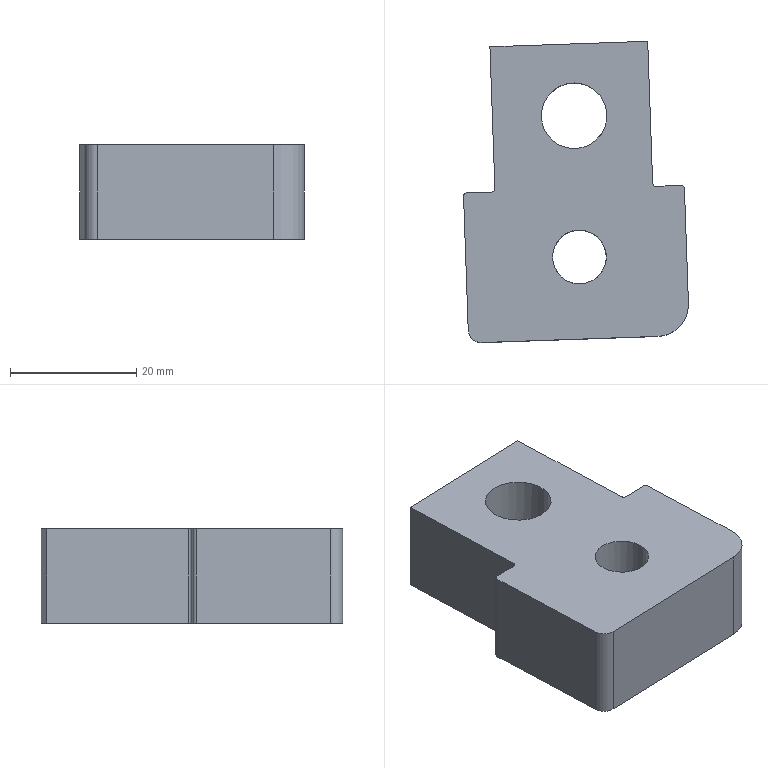Part | NX | features PS-30 2 | 1 solid | 18 faces | box 35.619 x 47.713 x 15 mm | volume 18881 mm3 | plane 10 | cylinder 8 | commonest cylinder face diameters 1 x4 4 x1 8.506 x1 10 x1 10.4 x1
STEP:
#1=CARTESIAN_POINT('',(3332.266,-814.738,900.716));
#2=VERTEX_POINT('',#1);
#3=CARTESIAN_POINT('',(3332.266,-809.538,900.716));
#4=DIRECTION('',(0.,0.,1.));
#5=DIRECTION('',(0.,-1.,0.));
#6=AXIS2_PLACEMENT_3D('',#3,#4,#5);
#7=CIRCLE('',#6,5.2);
#8=EDGE_CURVE('',#2,#2,#7,.F.);
#9=ORIENTED_EDGE('',*,*,#8,.F.);
#10=EDGE_LOOP('',(#9));
#11=FACE_BOUND('',#10,.T.);
#12=CARTESIAN_POINT('',(3327.066,-809.538,885.716));
#13=VERTEX_POINT('',#12);
#14=CARTESIAN_POINT('',(3332.266,-809.538,885.716));
#15=DIRECTION('',(0.,0.,-1.));
#16=DIRECTION('',(-1.,0.,0.));
#17=AXIS2_PLACEMENT_3D('',#14,#15,#16);
#18=CIRCLE('',#17,5.2);
#19=EDGE_CURVE('',#13,#13,#18,.F.);
#20=ORIENTED_EDGE('',*,*,#19,.F.);
#21=EDGE_LOOP('',(#20));
#22=FACE_BOUND('',#21,.T.);
#23=CARTESIAN_POINT('',(3332.266,-809.538,890.716));
#24=DIRECTION('',(0.,0.,-1.));
#25=DIRECTION('',(0.9976,0.06975,0.));
#26=AXIS2_PLACEMENT_3D('',#23,#24,#25);
#27=CYLINDRICAL_SURFACE('',#26,5.2);
#28=ADVANCED_FACE('',(#11,#22),#27,.F.);
#29=CARTESIAN_POINT('',(3333.107,-836.157,900.716));
#30=VERTEX_POINT('',#29);
#31=CARTESIAN_POINT('',(3333.107,-831.904,900.716));
#32=DIRECTION('',(0.,0.,1.));
#33=DIRECTION('',(0.,-1.,0.));
#34=AXIS2_PLACEMENT_3D('',#31,#32,#33);
#35=CIRCLE('',#34,4.253);
#36=EDGE_CURVE('',#30,#30,#35,.F.);
#37=ORIENTED_EDGE('',*,*,#36,.F.);
#38=EDGE_LOOP('',(#37));
#39=FACE_BOUND('',#38,.T.);
#40=CARTESIAN_POINT('',(3328.854,-831.904,885.716));
#41=VERTEX_POINT('',#40);
#42=CARTESIAN_POINT('',(3333.107,-831.904,885.716));
#43=DIRECTION('',(0.,0.,-1.));
#44=DIRECTION('',(-1.,0.,0.));
#45=AXIS2_PLACEMENT_3D('',#42,#43,#44);
#46=CIRCLE('',#45,4.253);
#47=EDGE_CURVE('',#41,#41,#46,.T.);
#48=ORIENTED_EDGE('',*,*,#47,.T.);
#49=EDGE_LOOP('',(#48));
#50=FACE_BOUND('',#49,.T.);
#51=CARTESIAN_POINT('',(3333.107,-831.904,868.716));
#52=DIRECTION('',(0.,0.,1.));
#53=DIRECTION('',(0.9976,0.06975,0.));
#54=AXIS2_PLACEMENT_3D('',#51,#52,#53);
#55=CYLINDRICAL_SURFACE('',#54,4.253);
#56=ADVANCED_FACE('',(#39,#50),#55,.F.);
#57=ORIENTED_EDGE('',*,*,#36,.T.);
#58=EDGE_LOOP('',(#57));
#59=FACE_BOUND('',#58,.T.);
#60=CARTESIAN_POINT('',(3319.24,-821.618,900.716));
#61=VERTEX_POINT('',#60);
#62=CARTESIAN_POINT('',(3319.722,-821.101,900.716));
#63=VERTEX_POINT('',#62);
#64=CARTESIAN_POINT('',(3319.222,-821.119,900.716));
#65=DIRECTION('',(0.,0.,1.));
#66=DIRECTION('',(0.,-1.,0.));
#67=AXIS2_PLACEMENT_3D('',#64,#65,#66);
#68=CIRCLE('',#67,0.5);
#69=EDGE_CURVE('',#61,#63,#68,.T.);
#70=ORIENTED_EDGE('',*,*,#69,.F.);
#71=CARTESIAN_POINT('',(3315.242,-821.758,900.716));
#72=VERTEX_POINT('',#71);
#73=CARTESIAN_POINT('',(3173.832,-826.696,900.716));
#74=DIRECTION('',(0.9994,0.0349,0.));
#75=VECTOR('',#74,1000.);
#76=LINE('',#73,#75);
#77=EDGE_CURVE('',#61,#72,#76,.F.);
#78=ORIENTED_EDGE('',*,*,#77,.T.);
#79=CARTESIAN_POINT('',(3314.76,-822.275,900.716));
#80=VERTEX_POINT('',#79);
#81=CARTESIAN_POINT('',(3315.26,-822.258,900.716));
#82=DIRECTION('',(0.,0.,1.));
#83=DIRECTION('',(0.,-1.,0.));
#84=AXIS2_PLACEMENT_3D('',#81,#82,#83);
#85=CIRCLE('',#84,0.5);
#86=EDGE_CURVE('',#80,#72,#85,.F.);
#87=ORIENTED_EDGE('',*,*,#86,.F.);
#88=CARTESIAN_POINT('',(3315.502,-843.525,900.716));
#89=VERTEX_POINT('',#88);
#90=CARTESIAN_POINT('',(3312.834,-767.126,900.716));
#91=DIRECTION('',(-0.0349,0.9994,0.));
#92=VECTOR('',#91,1000.);
#93=LINE('',#90,#92);
#94=EDGE_CURVE('',#80,#89,#93,.F.);
#95=ORIENTED_EDGE('',*,*,#94,.T.);
#96=CARTESIAN_POINT('',(3317.57,-845.454,900.716));
#97=VERTEX_POINT('',#96);
#98=CARTESIAN_POINT('',(3317.501,-843.455,900.716));
#99=DIRECTION('',(0.,0.,1.));
#100=DIRECTION('',(0.,-1.,0.));
#101=AXIS2_PLACEMENT_3D('',#98,#99,#100);
#102=CIRCLE('',#101,2.);
#103=EDGE_CURVE('',#89,#97,#102,.T.);
#104=ORIENTED_EDGE('',*,*,#103,.T.);
#105=CARTESIAN_POINT('',(3345.553,-844.477,900.716));
#106=VERTEX_POINT('',#105);
#107=CARTESIAN_POINT('',(3174.662,-850.444,900.716));
#108=DIRECTION('',(-0.9994,-0.0349,0.));
#109=VECTOR('',#108,1000.);
#110=LINE('',#107,#109);
#111=EDGE_CURVE('',#106,#97,#110,.T.);
#112=ORIENTED_EDGE('',*,*,#111,.F.);
#113=CARTESIAN_POINT('',(3350.376,-839.306,900.716));
#114=VERTEX_POINT('',#113);
#115=CARTESIAN_POINT('',(3345.379,-839.48,900.716));
#116=DIRECTION('',(0.,0.,1.));
#117=DIRECTION('',(0.,-1.,0.));
#118=AXIS2_PLACEMENT_3D('',#115,#116,#117);
#119=CIRCLE('',#118,5.);
#120=EDGE_CURVE('',#106,#114,#119,.T.);
#121=ORIENTED_EDGE('',*,*,#120,.T.);
#122=CARTESIAN_POINT('',(3349.739,-821.054,900.716));
#123=VERTEX_POINT('',#122);
#124=CARTESIAN_POINT('',(3347.813,-765.904,900.716));
#125=DIRECTION('',(-0.0349,0.9994,0.));
#126=VECTOR('',#125,1000.);
#127=LINE('',#124,#126);
#128=EDGE_CURVE('',#123,#114,#127,.F.);
#129=ORIENTED_EDGE('',*,*,#128,.F.);
#130=CARTESIAN_POINT('',(3349.221,-820.572,900.716));
#131=VERTEX_POINT('',#130);
#132=CARTESIAN_POINT('',(3349.239,-821.071,900.716));
#133=DIRECTION('',(0.,0.,1.));
#134=DIRECTION('',(0.,-1.,0.));
#135=AXIS2_PLACEMENT_3D('',#132,#133,#134);
#136=CIRCLE('',#135,0.5);
#137=EDGE_CURVE('',#131,#123,#136,.F.);
#138=ORIENTED_EDGE('',*,*,#137,.F.);
#139=CARTESIAN_POINT('',(3345.224,-820.711,900.716));
#140=VERTEX_POINT('',#139);
#141=CARTESIAN_POINT('',(3173.832,-826.696,900.716));
#142=DIRECTION('',(0.9994,0.0349,0.));
#143=VECTOR('',#142,1000.);
#144=LINE('',#141,#143);
#145=EDGE_CURVE('',#131,#140,#144,.F.);
#146=ORIENTED_EDGE('',*,*,#145,.T.);
#147=CARTESIAN_POINT('',(3344.707,-820.229,900.716));
#148=VERTEX_POINT('',#147);
#149=CARTESIAN_POINT('',(3345.206,-820.211,900.716));
#150=DIRECTION('',(0.,0.,1.));
#151=DIRECTION('',(0.,-1.,0.));
#152=AXIS2_PLACEMENT_3D('',#149,#150,#151);
#153=CIRCLE('',#152,0.5);
#154=EDGE_CURVE('',#148,#140,#153,.T.);
#155=ORIENTED_EDGE('',*,*,#154,.F.);
#156=CARTESIAN_POINT('',(3343.922,-797.743,900.716));
#157=VERTEX_POINT('',#156);
#158=CARTESIAN_POINT('',(3342.816,-766.079,900.716));
#159=DIRECTION('',(-0.0349,0.9994,0.));
#160=VECTOR('',#159,1000.);
#161=LINE('',#158,#160);
#162=EDGE_CURVE('',#157,#148,#161,.F.);
#163=ORIENTED_EDGE('',*,*,#162,.F.);
#164=CARTESIAN_POINT('',(3318.937,-798.615,900.716));
#165=VERTEX_POINT('',#164);
#166=CARTESIAN_POINT('',(3328.742,-798.273,900.716));
#167=DIRECTION('',(-0.9994,-0.0349,0.));
#168=VECTOR('',#167,1000.);
#169=LINE('',#166,#168);
#170=EDGE_CURVE('',#157,#165,#169,.T.);
#171=ORIENTED_EDGE('',*,*,#170,.T.);
#172=CARTESIAN_POINT('',(3317.831,-766.951,900.716));
#173=DIRECTION('',(-0.0349,0.9994,0.));
#174=VECTOR('',#173,1000.);
#175=LINE('',#172,#174);
#176=EDGE_CURVE('',#165,#63,#175,.F.);
#177=ORIENTED_EDGE('',*,*,#176,.T.);
#178=EDGE_LOOP('',(#70,#78,#87,#95,#104,#112,#121,#129,#138,#146,#155,#163,#171,#177));
#179=FACE_BOUND('',#178,.T.);
#180=ORIENTED_EDGE('',*,*,#8,.T.);
#181=EDGE_LOOP('',(#180));
#182=FACE_BOUND('',#181,.T.);
#183=CARTESIAN_POINT('',(3171.924,-772.046,900.716));
#184=DIRECTION('',(0.,0.,1.));
#185=DIRECTION('',(0.9976,0.06975,0.));
#186=AXIS2_PLACEMENT_3D('',#183,#184,#185);
#187=PLANE('',#186);
#188=ADVANCED_FACE('',(#59,#179,#182),#187,.T.);
#189=CARTESIAN_POINT('',(3349.739,-821.054,885.716));
#190=VERTEX_POINT('',#189);
#191=CARTESIAN_POINT('',(3349.739,-821.054,868.716));
#192=DIRECTION('',(0.,0.,-1.));
#193=VECTOR('',#192,1000.);
#194=LINE('',#191,#193);
#195=EDGE_CURVE('',#123,#190,#194,.T.);
#196=ORIENTED_EDGE('',*,*,#195,.T.);
#197=CARTESIAN_POINT('',(3349.221,-820.572,885.716));
#198=VERTEX_POINT('',#197);
#199=CARTESIAN_POINT('',(3349.239,-821.071,885.716));
#200=DIRECTION('',(0.,0.,-1.));
#201=DIRECTION('',(-1.,0.,0.));
#202=AXIS2_PLACEMENT_3D('',#199,#200,#201);
#203=CIRCLE('',#202,0.5);
#204=EDGE_CURVE('',#190,#198,#203,.F.);
#205=ORIENTED_EDGE('',*,*,#204,.T.);
#206=CARTESIAN_POINT('',(3349.221,-820.572,890.716));
#207=DIRECTION('',(0.,0.,-1.));
#208=VECTOR('',#207,1000.);
#209=LINE('',#206,#208);
#210=EDGE_CURVE('',#198,#131,#209,.F.);
#211=ORIENTED_EDGE('',*,*,#210,.T.);
#212=ORIENTED_EDGE('',*,*,#137,.T.);
#213=EDGE_LOOP('',(#196,#205,#211,#212));
#214=FACE_BOUND('',#213,.T.);
#215=CARTESIAN_POINT('',(3349.239,-821.071,862.716));
#216=DIRECTION('',(0.,0.,1.));
#217=DIRECTION('',(1.,0.,0.));
#218=AXIS2_PLACEMENT_3D('',#215,#216,#217);
#219=CYLINDRICAL_SURFACE('',#218,0.5);
#220=ADVANCED_FACE('',(#214),#219,.T.);
#221=CARTESIAN_POINT('',(3345.553,-844.477,885.716));
#222=VERTEX_POINT('',#221);
#223=CARTESIAN_POINT('',(3345.553,-844.477,935.716));
#224=DIRECTION('',(0.,0.,-1.));
#225=VECTOR('',#224,1000.);
#226=LINE('',#223,#225);
#227=EDGE_CURVE('',#222,#106,#226,.F.);
#228=ORIENTED_EDGE('',*,*,#227,.F.);
#229=CARTESIAN_POINT('',(3350.376,-839.306,885.716));
#230=VERTEX_POINT('',#229);
#231=CARTESIAN_POINT('',(3345.379,-839.48,885.716));
#232=DIRECTION('',(0.,0.,-1.));
#233=DIRECTION('',(-1.,0.,0.));
#234=AXIS2_PLACEMENT_3D('',#231,#232,#233);
#235=CIRCLE('',#234,5.);
#236=EDGE_CURVE('',#230,#222,#235,.T.);
#237=ORIENTED_EDGE('',*,*,#236,.F.);
#238=CARTESIAN_POINT('',(3350.376,-839.306,862.716));
#239=DIRECTION('',(0.,0.,1.));
#240=VECTOR('',#239,1000.);
#241=LINE('',#238,#240);
#242=EDGE_CURVE('',#114,#230,#241,.F.);
#243=ORIENTED_EDGE('',*,*,#242,.F.);
#244=ORIENTED_EDGE('',*,*,#120,.F.);
#245=EDGE_LOOP('',(#228,#237,#243,#244));
#246=FACE_BOUND('',#245,.T.);
#247=CARTESIAN_POINT('',(3345.379,-839.48,862.716));
#248=DIRECTION('',(0.,0.,1.));
#249=DIRECTION('',(0.9976,0.06975,0.));
#250=AXIS2_PLACEMENT_3D('',#247,#248,#249);
#251=CYLINDRICAL_SURFACE('',#250,5.);
#252=ADVANCED_FACE('',(#246),#251,.T.);
#253=CARTESIAN_POINT('',(3315.242,-821.758,885.716));
#254=VERTEX_POINT('',#253);
#255=CARTESIAN_POINT('',(3315.242,-821.758,863.216));
#256=DIRECTION('',(0.,0.,1.));
#257=VECTOR('',#256,1000.);
#258=LINE('',#255,#257);
#259=EDGE_CURVE('',#72,#254,#258,.F.);
#260=ORIENTED_EDGE('',*,*,#259,.T.);
#261=CARTESIAN_POINT('',(3314.76,-822.275,885.716));
#262=VERTEX_POINT('',#261);
#263=CARTESIAN_POINT('',(3315.26,-822.258,885.716));
#264=DIRECTION('',(0.,0.,-1.));
#265=DIRECTION('',(-1.,0.,0.));
#266=AXIS2_PLACEMENT_3D('',#263,#264,#265);
#267=CIRCLE('',#266,0.5);
#268=EDGE_CURVE('',#262,#254,#267,.T.);
#269=ORIENTED_EDGE('',*,*,#268,.F.);
#270=CARTESIAN_POINT('',(3314.76,-822.275,890.716));
#271=DIRECTION('',(0.,0.,1.));
#272=VECTOR('',#271,1000.);
#273=LINE('',#270,#272);
#274=EDGE_CURVE('',#262,#80,#273,.T.);
#275=ORIENTED_EDGE('',*,*,#274,.T.);
#276=ORIENTED_EDGE('',*,*,#86,.T.);
#277=EDGE_LOOP('',(#260,#269,#275,#276));
#278=FACE_BOUND('',#277,.T.);
#279=CARTESIAN_POINT('',(3315.26,-822.258,890.716));
#280=DIRECTION('',(0.,0.,1.));
#281=DIRECTION('',(1.,0.,0.));
#282=AXIS2_PLACEMENT_3D('',#279,#280,#281);
#283=CYLINDRICAL_SURFACE('',#282,0.5);
#284=ADVANCED_FACE('',(#278),#283,.T.);
#285=CARTESIAN_POINT('',(3315.502,-843.525,885.716));
#286=VERTEX_POINT('',#285);
#287=CARTESIAN_POINT('',(3315.502,-843.525,890.716));
#288=DIRECTION('',(0.,0.,1.));
#289=VECTOR('',#288,1000.);
#290=LINE('',#287,#289);
#291=EDGE_CURVE('',#286,#89,#290,.T.);
#292=ORIENTED_EDGE('',*,*,#291,.F.);
#293=CARTESIAN_POINT('',(3317.57,-845.454,885.716));
#294=VERTEX_POINT('',#293);
#295=CARTESIAN_POINT('',(3317.501,-843.455,885.716));
#296=DIRECTION('',(0.,0.,-1.));
#297=DIRECTION('',(-1.,0.,0.));
#298=AXIS2_PLACEMENT_3D('',#295,#296,#297);
#299=CIRCLE('',#298,2.);
#300=EDGE_CURVE('',#286,#294,#299,.F.);
#301=ORIENTED_EDGE('',*,*,#300,.T.);
#302=CARTESIAN_POINT('',(3317.57,-845.454,860.716));
#303=DIRECTION('',(0.,0.,-1.));
#304=VECTOR('',#303,1000.);
#305=LINE('',#302,#304);
#306=EDGE_CURVE('',#97,#294,#305,.T.);
#307=ORIENTED_EDGE('',*,*,#306,.F.);
#308=ORIENTED_EDGE('',*,*,#103,.F.);
#309=EDGE_LOOP('',(#292,#301,#307,#308));
#310=FACE_BOUND('',#309,.T.);
#311=CARTESIAN_POINT('',(3317.501,-843.455,935.716));
#312=DIRECTION('',(0.,0.,-1.));
#313=DIRECTION('',(-0.9976,-0.06975,0.));
#314=AXIS2_PLACEMENT_3D('',#311,#312,#313);
#315=CYLINDRICAL_SURFACE('',#314,2.);
#316=ADVANCED_FACE('',(#310),#315,.T.);
#317=CARTESIAN_POINT('',(3314.523,-815.501,885.716));
#318=DIRECTION('',(-0.0349,0.9994,0.));
#319=VECTOR('',#318,1000.);
#320=LINE('',#317,#319);
#321=EDGE_CURVE('',#262,#286,#320,.F.);
#322=ORIENTED_EDGE('',*,*,#321,.T.);
#323=ORIENTED_EDGE('',*,*,#291,.T.);
#324=ORIENTED_EDGE('',*,*,#94,.F.);
#325=ORIENTED_EDGE('',*,*,#274,.F.);
#326=EDGE_LOOP('',(#322,#323,#324,#325));
#327=FACE_BOUND('',#326,.T.);
#328=CARTESIAN_POINT('',(3314.523,-815.501,890.716));
#329=DIRECTION('',(0.9994,0.0349,0.));
#330=DIRECTION('',(-0.0349,0.9994,0.));
#331=AXIS2_PLACEMENT_3D('',#328,#329,#330);
#332=PLANE('',#331);
#333=ADVANCED_FACE('',(#327),#332,.F.);
#334=ORIENTED_EDGE('',*,*,#306,.T.);
#335=CARTESIAN_POINT('',(3304.578,-845.908,885.716));
#336=DIRECTION('',(-0.9994,-0.0349,0.));
#337=VECTOR('',#336,1000.);
#338=LINE('',#335,#337);
#339=EDGE_CURVE('',#222,#294,#338,.T.);
#340=ORIENTED_EDGE('',*,*,#339,.F.);
#341=ORIENTED_EDGE('',*,*,#227,.T.);
#342=ORIENTED_EDGE('',*,*,#111,.T.);
#343=EDGE_LOOP('',(#334,#340,#341,#342));
#344=FACE_BOUND('',#343,.T.);
#345=CARTESIAN_POINT('',(3304.578,-845.908,935.716));
#346=DIRECTION('',(-0.0349,0.9994,0.));
#347=DIRECTION('',(-0.9994,-0.0349,0.));
#348=AXIS2_PLACEMENT_3D('',#345,#346,#347);
#349=PLANE('',#348);
#350=ADVANCED_FACE('',(#344),#349,.F.);
#351=ORIENTED_EDGE('',*,*,#242,.T.);
#352=CARTESIAN_POINT('',(3349.537,-815.279,885.716));
#353=DIRECTION('',(-0.0349,0.9994,0.));
#354=VECTOR('',#353,1000.);
#355=LINE('',#352,#354);
#356=EDGE_CURVE('',#230,#190,#355,.T.);
#357=ORIENTED_EDGE('',*,*,#356,.T.);
#358=ORIENTED_EDGE('',*,*,#195,.F.);
#359=ORIENTED_EDGE('',*,*,#128,.T.);
#360=EDGE_LOOP('',(#351,#357,#358,#359));
#361=FACE_BOUND('',#360,.T.);
#362=CARTESIAN_POINT('',(3349.537,-815.279,862.716));
#363=DIRECTION('',(0.9994,0.0349,0.));
#364=DIRECTION('',(-0.0349,0.9994,0.));
#365=AXIS2_PLACEMENT_3D('',#362,#363,#364);
#366=PLANE('',#365);
#367=ADVANCED_FACE('',(#361),#366,.T.);
#368=CARTESIAN_POINT('',(3345.224,-820.711,885.716));
#369=VERTEX_POINT('',#368);
#370=CARTESIAN_POINT('',(3329.542,-821.259,885.716));
#371=DIRECTION('',(0.9994,0.0349,0.));
#372=VECTOR('',#371,1000.);
#373=LINE('',#370,#372);
#374=EDGE_CURVE('',#369,#198,#373,.T.);
#375=ORIENTED_EDGE('',*,*,#374,.F.);
#376=CARTESIAN_POINT('',(3345.224,-820.711,863.216));
#377=DIRECTION('',(0.,0.,1.));
#378=VECTOR('',#377,1000.);
#379=LINE('',#376,#378);
#380=EDGE_CURVE('',#140,#369,#379,.F.);
#381=ORIENTED_EDGE('',*,*,#380,.F.);
#382=ORIENTED_EDGE('',*,*,#145,.F.);
#383=ORIENTED_EDGE('',*,*,#210,.F.);
#384=EDGE_LOOP('',(#375,#381,#382,#383));
#385=FACE_BOUND('',#384,.T.);
#386=CARTESIAN_POINT('',(3329.542,-821.259,863.216));
#387=DIRECTION('',(0.0349,-0.9994,0.));
#388=DIRECTION('',(-0.9994,-0.0349,0.));
#389=AXIS2_PLACEMENT_3D('',#386,#387,#388);
#390=PLANE('',#389);
#391=ADVANCED_FACE('',(#385),#390,.F.);
#392=CARTESIAN_POINT('',(3319.24,-821.618,885.716));
#393=VERTEX_POINT('',#392);
#394=CARTESIAN_POINT('',(3329.542,-821.259,885.716));
#395=DIRECTION('',(0.9994,0.0349,0.));
#396=VECTOR('',#395,1000.);
#397=LINE('',#394,#396);
#398=EDGE_CURVE('',#254,#393,#397,.T.);
#399=ORIENTED_EDGE('',*,*,#398,.F.);
#400=ORIENTED_EDGE('',*,*,#259,.F.);
#401=ORIENTED_EDGE('',*,*,#77,.F.);
#402=CARTESIAN_POINT('',(3319.24,-821.618,890.716));
#403=DIRECTION('',(0.,0.,-1.));
#404=VECTOR('',#403,1000.);
#405=LINE('',#402,#404);
#406=EDGE_CURVE('',#393,#61,#405,.F.);
#407=ORIENTED_EDGE('',*,*,#406,.F.);
#408=EDGE_LOOP('',(#399,#400,#401,#407));
#409=FACE_BOUND('',#408,.T.);
#410=CARTESIAN_POINT('',(3329.542,-821.259,863.216));
#411=DIRECTION('',(0.0349,-0.9994,0.));
#412=DIRECTION('',(-0.9994,-0.0349,0.));
#413=AXIS2_PLACEMENT_3D('',#410,#411,#412);
#414=PLANE('',#413);
#415=ADVANCED_FACE('',(#409),#414,.F.);
#416=CARTESIAN_POINT('',(3344.707,-820.229,885.716));
#417=VERTEX_POINT('',#416);
#418=CARTESIAN_POINT('',(3345.206,-820.211,885.716));
#419=DIRECTION('',(0.,0.,-1.));
#420=DIRECTION('',(-1.,0.,0.));
#421=AXIS2_PLACEMENT_3D('',#418,#419,#420);
#422=CIRCLE('',#421,0.5);
#423=EDGE_CURVE('',#369,#417,#422,.T.);
#424=ORIENTED_EDGE('',*,*,#423,.T.);
#425=CARTESIAN_POINT('',(3344.707,-820.229,862.716));
#426=DIRECTION('',(0.,0.,1.));
#427=VECTOR('',#426,1000.);
#428=LINE('',#425,#427);
#429=EDGE_CURVE('',#417,#148,#428,.T.);
#430=ORIENTED_EDGE('',*,*,#429,.T.);
#431=ORIENTED_EDGE('',*,*,#154,.T.);
#432=ORIENTED_EDGE('',*,*,#380,.T.);
#433=EDGE_LOOP('',(#424,#430,#431,#432));
#434=FACE_BOUND('',#433,.T.);
#435=CARTESIAN_POINT('',(3345.206,-820.211,862.716));
#436=DIRECTION('',(0.,0.,1.));
#437=DIRECTION('',(1.,0.,0.));
#438=AXIS2_PLACEMENT_3D('',#435,#436,#437);
#439=CYLINDRICAL_SURFACE('',#438,0.5);
#440=ADVANCED_FACE('',(#434),#439,.F.);
#441=CARTESIAN_POINT('',(3319.722,-821.101,885.716));
#442=VERTEX_POINT('',#441);
#443=CARTESIAN_POINT('',(3319.222,-821.119,885.716));
#444=DIRECTION('',(0.,0.,-1.));
#445=DIRECTION('',(-1.,0.,0.));
#446=AXIS2_PLACEMENT_3D('',#443,#444,#445);
#447=CIRCLE('',#446,0.5);
#448=EDGE_CURVE('',#442,#393,#447,.T.);
#449=ORIENTED_EDGE('',*,*,#448,.T.);
#450=ORIENTED_EDGE('',*,*,#406,.T.);
#451=ORIENTED_EDGE('',*,*,#69,.T.);
#452=CARTESIAN_POINT('',(3319.722,-821.101,868.716));
#453=DIRECTION('',(0.,0.,-1.));
#454=VECTOR('',#453,1000.);
#455=LINE('',#452,#454);
#456=EDGE_CURVE('',#63,#442,#455,.T.);
#457=ORIENTED_EDGE('',*,*,#456,.T.);
#458=EDGE_LOOP('',(#449,#450,#451,#457));
#459=FACE_BOUND('',#458,.T.);
#460=CARTESIAN_POINT('',(3319.222,-821.119,890.716));
#461=DIRECTION('',(0.,0.,1.));
#462=DIRECTION('',(1.,0.,0.));
#463=AXIS2_PLACEMENT_3D('',#460,#461,#462);
#464=CYLINDRICAL_SURFACE('',#463,0.5);
#465=ADVANCED_FACE('',(#459),#464,.F.);
#466=ORIENTED_EDGE('',*,*,#429,.F.);
#467=CARTESIAN_POINT('',(3343.922,-797.743,885.716));
#468=VERTEX_POINT('',#467);
#469=CARTESIAN_POINT('',(3344.54,-815.453,885.716));
#470=DIRECTION('',(-0.0349,0.9994,0.));
#471=VECTOR('',#470,1000.);
#472=LINE('',#469,#471);
#473=EDGE_CURVE('',#468,#417,#472,.F.);
#474=ORIENTED_EDGE('',*,*,#473,.F.);
#475=CARTESIAN_POINT('',(3343.922,-797.743,862.716));
#476=DIRECTION('',(0.,0.,-1.));
#477=VECTOR('',#476,1000.);
#478=LINE('',#475,#477);
#479=EDGE_CURVE('',#468,#157,#478,.F.);
#480=ORIENTED_EDGE('',*,*,#479,.T.);
#481=ORIENTED_EDGE('',*,*,#162,.T.);
#482=EDGE_LOOP('',(#466,#474,#480,#481));
#483=FACE_BOUND('',#482,.T.);
#484=CARTESIAN_POINT('',(3344.54,-815.453,862.716));
#485=DIRECTION('',(0.9994,0.0349,0.));
#486=DIRECTION('',(-0.0349,0.9994,0.));
#487=AXIS2_PLACEMENT_3D('',#484,#485,#486);
#488=PLANE('',#487);
#489=ADVANCED_FACE('',(#483),#488,.T.);
#490=ORIENTED_EDGE('',*,*,#479,.F.);
#491=CARTESIAN_POINT('',(3318.937,-798.615,885.716));
#492=VERTEX_POINT('',#491);
#493=CARTESIAN_POINT('',(3328.742,-798.273,885.716));
#494=DIRECTION('',(0.9994,0.0349,0.));
#495=VECTOR('',#494,1000.);
#496=LINE('',#493,#495);
#497=EDGE_CURVE('',#468,#492,#496,.F.);
#498=ORIENTED_EDGE('',*,*,#497,.T.);
#499=CARTESIAN_POINT('',(3318.937,-798.615,863.216));
#500=DIRECTION('',(0.,0.,1.));
#501=VECTOR('',#500,1000.);
#502=LINE('',#499,#501);
#503=EDGE_CURVE('',#165,#492,#502,.F.);
#504=ORIENTED_EDGE('',*,*,#503,.F.);
#505=ORIENTED_EDGE('',*,*,#170,.F.);
#506=EDGE_LOOP('',(#490,#498,#504,#505));
#507=FACE_BOUND('',#506,.T.);
#508=CARTESIAN_POINT('',(3328.742,-798.273,863.216));
#509=DIRECTION('',(0.0349,-0.9994,0.));
#510=DIRECTION('',(-0.9994,-0.0349,0.));
#511=AXIS2_PLACEMENT_3D('',#508,#509,#510);
#512=PLANE('',#511);
#513=ADVANCED_FACE('',(#507),#512,.F.);
#514=CARTESIAN_POINT('',(3319.52,-815.326,885.716));
#515=DIRECTION('',(-0.0349,0.9994,0.));
#516=VECTOR('',#515,1000.);
#517=LINE('',#514,#516);
#518=EDGE_CURVE('',#442,#492,#517,.T.);
#519=ORIENTED_EDGE('',*,*,#518,.F.);
#520=ORIENTED_EDGE('',*,*,#456,.F.);
#521=ORIENTED_EDGE('',*,*,#176,.F.);
#522=ORIENTED_EDGE('',*,*,#503,.T.);
#523=EDGE_LOOP('',(#519,#520,#521,#522));
#524=FACE_BOUND('',#523,.T.);
#525=CARTESIAN_POINT('',(3319.52,-815.326,890.716));
#526=DIRECTION('',(0.9994,0.0349,0.));
#527=DIRECTION('',(-0.0349,0.9994,0.));
#528=AXIS2_PLACEMENT_3D('',#525,#526,#527);
#529=PLANE('',#528);
#530=ADVANCED_FACE('',(#524),#529,.F.);
#531=ORIENTED_EDGE('',*,*,#47,.F.);
#532=EDGE_LOOP('',(#531));
#533=FACE_BOUND('',#532,.T.);
#534=ORIENTED_EDGE('',*,*,#473,.T.);
#535=ORIENTED_EDGE('',*,*,#423,.F.);
#536=ORIENTED_EDGE('',*,*,#374,.T.);
#537=ORIENTED_EDGE('',*,*,#204,.F.);
#538=ORIENTED_EDGE('',*,*,#356,.F.);
#539=ORIENTED_EDGE('',*,*,#236,.T.);
#540=ORIENTED_EDGE('',*,*,#339,.T.);
#541=ORIENTED_EDGE('',*,*,#300,.F.);
#542=ORIENTED_EDGE('',*,*,#321,.F.);
#543=ORIENTED_EDGE('',*,*,#268,.T.);
#544=ORIENTED_EDGE('',*,*,#398,.T.);
#545=ORIENTED_EDGE('',*,*,#448,.F.);
#546=ORIENTED_EDGE('',*,*,#518,.T.);
#547=ORIENTED_EDGE('',*,*,#497,.F.);
#548=EDGE_LOOP('',(#534,#535,#536,#537,#538,#539,#540,#541,#542,#543,#544,#545,#546,#547));
#549=FACE_BOUND('',#548,.T.);
#550=ORIENTED_EDGE('',*,*,#19,.T.);
#551=EDGE_LOOP('',(#550));
#552=FACE_BOUND('',#551,.T.);
#553=CARTESIAN_POINT('',(3332.569,-833.013,885.716));
#554=DIRECTION('',(0.,0.,-1.));
#555=DIRECTION('',(-1.,0.,0.));
#556=AXIS2_PLACEMENT_3D('',#553,#554,#555);
#557=PLANE('',#556);
#558=ADVANCED_FACE('',(#533,#549,#552),#557,.T.);
#559=CLOSED_SHELL('',(#28,#56,#188,#220,#252,#284,#316,#333,#350,#367,#391,#415,#440,#465,#489,#513,#530,#558));
#560=MANIFOLD_SOLID_BREP('',#559);
#561=(LENGTH_UNIT()NAMED_UNIT(*)SI_UNIT(.MILLI.,.METRE.));
#562=UNCERTAINTY_MEASURE_WITH_UNIT(LENGTH_MEASURE(0.00001),#561,'','');
#563=(NAMED_UNIT(*)PLANE_ANGLE_UNIT()SI_UNIT($,.RADIAN.));
#564=(NAMED_UNIT(*)SI_UNIT($,.STERADIAN.)SOLID_ANGLE_UNIT());
#565=(GEOMETRIC_REPRESENTATION_CONTEXT(3)GLOBAL_UNCERTAINTY_ASSIGNED_CONTEXT((#562))GLOBAL_UNIT_ASSIGNED_CONTEXT((#561,#563,#564))REPRESENTATION_CONTEXT('',''));
#566=ADVANCED_BREP_SHAPE_REPRESENTATION('',(#560),#565);